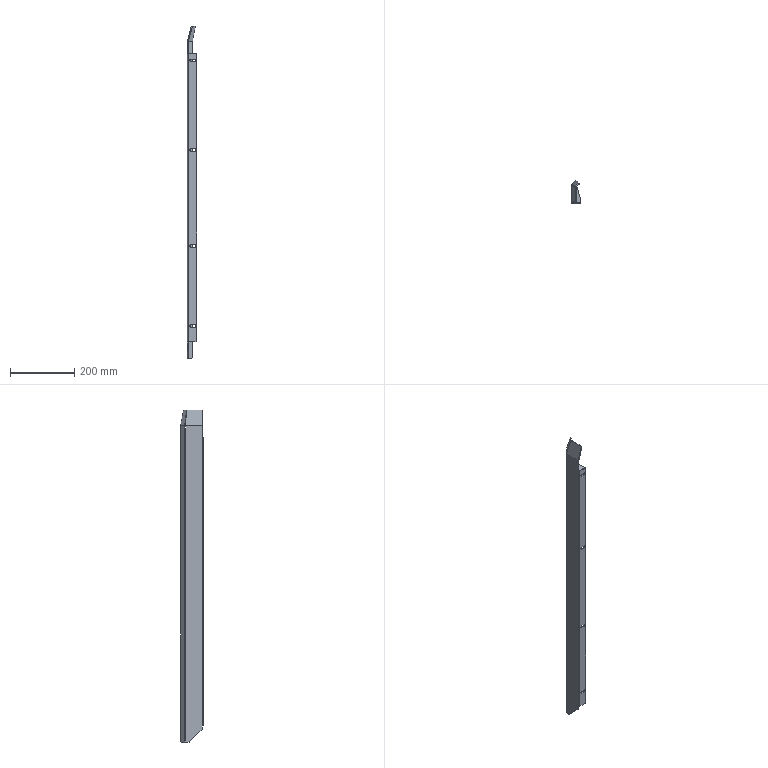Part | STEP file | KF-2212-070-004 | 4 solids | 87 faces | box 30 x 71.142 x 1037 mm | volume 309462 mm3 | plane 62 | cylinder 23 | spline 2 | commonest cylinder face diameters 7 x12 5 x7 1 x4